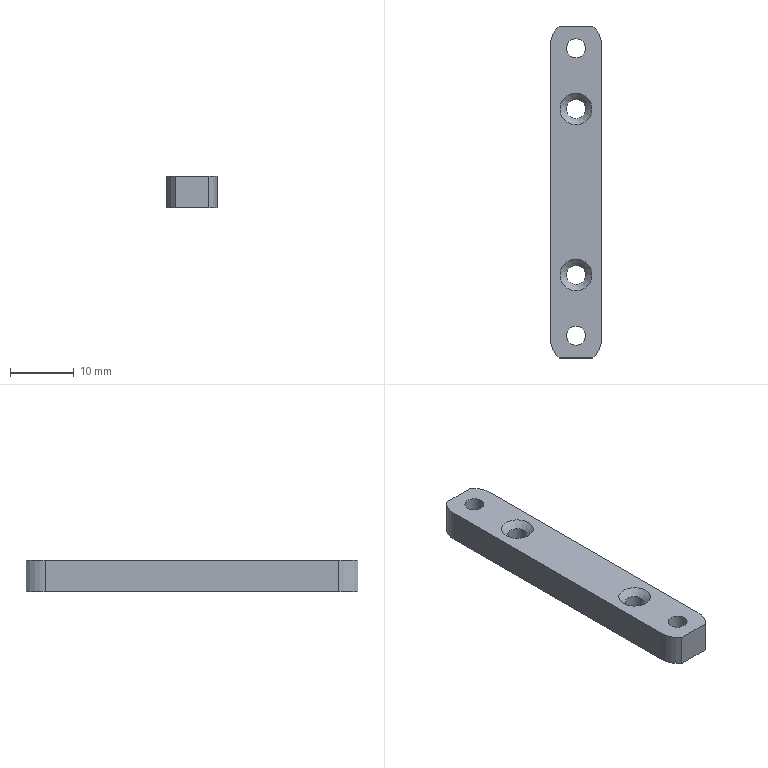Part | STEP file | Wytnij-wyci_gni_cie1_1 | 1 solid | 16 faces | box 8 x 52 x 5 mm | volume 1902 mm3 | cylinder 8 | plane 6 | cone 2 | commonest cylinder face diameters 3 x4 7.98 x4
STEP:
#1=CARTESIAN_POINT('',(0.,0.,0.));
#2=DIRECTION('',(0.,0.,1.));
#3=DIRECTION('',(1.,0.,0.));
#4=AXIS2_PLACEMENT_3D('',#1,#2,#3);
#5=CARTESIAN_POINT('',(-65.244,65.807,-118.498));
#6=VERTEX_POINT('',#5);
#7=CARTESIAN_POINT('',(-63.744,65.807,-118.498));
#8=DIRECTION('',(0.,0.,-1.));
#9=DIRECTION('',(-1.,0.,0.));
#10=AXIS2_PLACEMENT_3D('',#7,#8,#9);
#11=CIRCLE('',#10,1.5);
#12=CARTESIAN_POINT('',(-63.744,65.807,-118.498));
#13=DIRECTION('',(0.,0.,-1.));
#14=DIRECTION('',(-1.,0.,0.));
#15=AXIS2_PLACEMENT_3D('',#12,#13,#14);
#16=CYLINDRICAL_SURFACE('',#15,1.5);
#17=CARTESIAN_POINT('',(0.,0.));
#18=DIRECTION('',(1.,0.));
#19=VECTOR('',#18,1.);
#20=LINE('',#17,#19);
#21=(GEOMETRIC_REPRESENTATION_CONTEXT(2)PARAMETRIC_REPRESENTATION_CONTEXT()REPRESENTATION_CONTEXT('',''));
#22=DEFINITIONAL_REPRESENTATION('',(#20),#21);
#23=PCURVE('',#16,#22);
#24=CARTESIAN_POINT('',(-63.744,88.307,-118.498));
#25=DIRECTION('',(0.,0.,1.));
#26=DIRECTION('',(1.,0.,0.));
#27=AXIS2_PLACEMENT_3D('',#24,#25,#26);
#28=PLANE('',#27);
#29=CARTESIAN_POINT('',(-1.5,-22.5));
#30=CARTESIAN_POINT('',(-1.5,-19.902));
#31=CARTESIAN_POINT('',(0.75,-21.201));
#32=CARTESIAN_POINT('',(3.,-22.5));
#33=CARTESIAN_POINT('',(0.75,-23.799));
#34=CARTESIAN_POINT('',(-1.5,-25.098));
#35=CARTESIAN_POINT('',(-1.5,-22.5));
#36=(BOUNDED_CURVE()B_SPLINE_CURVE(2,(#29,#30,#31,#32,#33,#34,#35),.UNSPECIFIED.,.T.,.F.)B_SPLINE_CURVE_WITH_KNOTS((1,2,2,2,2,1),(-2.094,0.,2.094,4.189,6.283,8.378),.UNSPECIFIED.)CURVE()GEOMETRIC_REPRESENTATION_ITEM()RATIONAL_B_SPLINE_CURVE((1.,0.5,1.,0.5,1.,0.5,1.))REPRESENTATION_ITEM(''));
#37=(GEOMETRIC_REPRESENTATION_CONTEXT(2)PARAMETRIC_REPRESENTATION_CONTEXT()REPRESENTATION_CONTEXT('',''));
#38=DEFINITIONAL_REPRESENTATION('',(#36),#37);
#39=PCURVE('',#28,#38);
#40=SURFACE_CURVE('',#11,(#23,#39),.PCURVE_S1.);
#41=EDGE_CURVE('',#6,#6,#40,.T.);
#42=ORIENTED_EDGE('',*,*,#41,.T.);
#43=CARTESIAN_POINT('',(-65.244,65.807,-123.498));
#44=VERTEX_POINT('',#43);
#45=CARTESIAN_POINT('',(-65.244,65.807,-123.498));
#46=DIRECTION('',(0.,0.,1.));
#47=VECTOR('',#46,1.);
#48=LINE('',#45,#47);
#49=CARTESIAN_POINT('',(6.283,5.));
#50=DIRECTION('',(0.,-1.));
#51=VECTOR('',#50,1.);
#52=LINE('',#49,#51);
#53=(GEOMETRIC_REPRESENTATION_CONTEXT(2)PARAMETRIC_REPRESENTATION_CONTEXT()REPRESENTATION_CONTEXT('',''));
#54=DEFINITIONAL_REPRESENTATION('',(#52),#53);
#55=PCURVE('',#16,#54);
#56=CARTESIAN_POINT('',(0.,5.));
#57=DIRECTION('',(0.,-1.));
#58=VECTOR('',#57,1.);
#59=LINE('',#56,#58);
#60=(GEOMETRIC_REPRESENTATION_CONTEXT(2)PARAMETRIC_REPRESENTATION_CONTEXT()REPRESENTATION_CONTEXT('',''));
#61=DEFINITIONAL_REPRESENTATION('',(#59),#60);
#62=PCURVE('',#16,#61);
#63=SEAM_CURVE('',#48,(#55,#62),.PCURVE_S1.);
#64=EDGE_CURVE('',#44,#6,#63,.T.);
#65=ORIENTED_EDGE('',*,*,#64,.F.);
#66=CARTESIAN_POINT('',(-63.744,65.807,-123.498));
#67=DIRECTION('',(0.,0.,-1.));
#68=DIRECTION('',(-1.,0.,0.));
#69=AXIS2_PLACEMENT_3D('',#66,#67,#68);
#70=CIRCLE('',#69,1.5);
#71=CARTESIAN_POINT('',(0.,5.));
#72=DIRECTION('',(1.,0.));
#73=VECTOR('',#72,1.);
#74=LINE('',#71,#73);
#75=(GEOMETRIC_REPRESENTATION_CONTEXT(2)PARAMETRIC_REPRESENTATION_CONTEXT()REPRESENTATION_CONTEXT('',''));
#76=DEFINITIONAL_REPRESENTATION('',(#74),#75);
#77=PCURVE('',#16,#76);
#78=CARTESIAN_POINT('',(-63.744,88.307,-123.498));
#79=DIRECTION('',(0.,0.,1.));
#80=DIRECTION('',(1.,0.,0.));
#81=AXIS2_PLACEMENT_3D('',#78,#79,#80);
#82=PLANE('',#81);
#83=CARTESIAN_POINT('',(-1.5,-22.5));
#84=CARTESIAN_POINT('',(-1.5,-19.902));
#85=CARTESIAN_POINT('',(0.75,-21.201));
#86=CARTESIAN_POINT('',(3.,-22.5));
#87=CARTESIAN_POINT('',(0.75,-23.799));
#88=CARTESIAN_POINT('',(-1.5,-25.098));
#89=CARTESIAN_POINT('',(-1.5,-22.5));
#90=(BOUNDED_CURVE()B_SPLINE_CURVE(2,(#83,#84,#85,#86,#87,#88,#89),.UNSPECIFIED.,.T.,.F.)B_SPLINE_CURVE_WITH_KNOTS((1,2,2,2,2,1),(-2.094,0.,2.094,4.189,6.283,8.378),.UNSPECIFIED.)CURVE()GEOMETRIC_REPRESENTATION_ITEM()RATIONAL_B_SPLINE_CURVE((1.,0.5,1.,0.5,1.,0.5,1.))REPRESENTATION_ITEM(''));
#91=(GEOMETRIC_REPRESENTATION_CONTEXT(2)PARAMETRIC_REPRESENTATION_CONTEXT()REPRESENTATION_CONTEXT('',''));
#92=DEFINITIONAL_REPRESENTATION('',(#90),#91);
#93=PCURVE('',#82,#92);
#94=SURFACE_CURVE('',#70,(#77,#93),.PCURVE_S1.);
#95=EDGE_CURVE('',#44,#44,#94,.T.);
#96=ORIENTED_EDGE('',*,*,#95,.F.);
#97=ORIENTED_EDGE('',*,*,#64,.T.);
#98=EDGE_LOOP('',(#42,#65,#96,#97));
#99=FACE_BOUND('',#98,.F.);
#100=ADVANCED_FACE('',(#99),#16,.F.);
#101=CARTESIAN_POINT('',(-65.244,110.807,-118.498));
#102=VERTEX_POINT('',#101);
#103=CARTESIAN_POINT('',(-63.744,110.807,-118.498));
#104=DIRECTION('',(0.,0.,-1.));
#105=DIRECTION('',(-1.,0.,0.));
#106=AXIS2_PLACEMENT_3D('',#103,#104,#105);
#107=CIRCLE('',#106,1.5);
#108=CARTESIAN_POINT('',(-63.744,110.807,-118.498));
#109=DIRECTION('',(0.,0.,-1.));
#110=DIRECTION('',(-1.,0.,0.));
#111=AXIS2_PLACEMENT_3D('',#108,#109,#110);
#112=CYLINDRICAL_SURFACE('',#111,1.5);
#113=CARTESIAN_POINT('',(0.,0.));
#114=DIRECTION('',(1.,0.));
#115=VECTOR('',#114,1.);
#116=LINE('',#113,#115);
#117=(GEOMETRIC_REPRESENTATION_CONTEXT(2)PARAMETRIC_REPRESENTATION_CONTEXT()REPRESENTATION_CONTEXT('',''));
#118=DEFINITIONAL_REPRESENTATION('',(#116),#117);
#119=PCURVE('',#112,#118);
#120=CARTESIAN_POINT('',(-1.5,22.5));
#121=CARTESIAN_POINT('',(-1.5,25.098));
#122=CARTESIAN_POINT('',(0.75,23.799));
#123=CARTESIAN_POINT('',(3.,22.5));
#124=CARTESIAN_POINT('',(0.75,21.201));
#125=CARTESIAN_POINT('',(-1.5,19.902));
#126=CARTESIAN_POINT('',(-1.5,22.5));
#127=(BOUNDED_CURVE()B_SPLINE_CURVE(2,(#120,#121,#122,#123,#124,#125,#126),.UNSPECIFIED.,.T.,.F.)B_SPLINE_CURVE_WITH_KNOTS((1,2,2,2,2,1),(-2.094,0.,2.094,4.189,6.283,8.378),.UNSPECIFIED.)CURVE()GEOMETRIC_REPRESENTATION_ITEM()RATIONAL_B_SPLINE_CURVE((1.,0.5,1.,0.5,1.,0.5,1.))REPRESENTATION_ITEM(''));
#128=(GEOMETRIC_REPRESENTATION_CONTEXT(2)PARAMETRIC_REPRESENTATION_CONTEXT()REPRESENTATION_CONTEXT('',''));
#129=DEFINITIONAL_REPRESENTATION('',(#127),#128);
#130=PCURVE('',#28,#129);
#131=SURFACE_CURVE('',#107,(#119,#130),.PCURVE_S1.);
#132=EDGE_CURVE('',#102,#102,#131,.T.);
#133=ORIENTED_EDGE('',*,*,#132,.T.);
#134=CARTESIAN_POINT('',(-65.244,110.807,-123.498));
#135=VERTEX_POINT('',#134);
#136=CARTESIAN_POINT('',(-65.244,110.807,-123.498));
#137=DIRECTION('',(0.,0.,1.));
#138=VECTOR('',#137,1.);
#139=LINE('',#136,#138);
#140=CARTESIAN_POINT('',(6.283,5.));
#141=DIRECTION('',(0.,-1.));
#142=VECTOR('',#141,1.);
#143=LINE('',#140,#142);
#144=(GEOMETRIC_REPRESENTATION_CONTEXT(2)PARAMETRIC_REPRESENTATION_CONTEXT()REPRESENTATION_CONTEXT('',''));
#145=DEFINITIONAL_REPRESENTATION('',(#143),#144);
#146=PCURVE('',#112,#145);
#147=CARTESIAN_POINT('',(0.,5.));
#148=DIRECTION('',(0.,-1.));
#149=VECTOR('',#148,1.);
#150=LINE('',#147,#149);
#151=(GEOMETRIC_REPRESENTATION_CONTEXT(2)PARAMETRIC_REPRESENTATION_CONTEXT()REPRESENTATION_CONTEXT('',''));
#152=DEFINITIONAL_REPRESENTATION('',(#150),#151);
#153=PCURVE('',#112,#152);
#154=SEAM_CURVE('',#139,(#146,#153),.PCURVE_S1.);
#155=EDGE_CURVE('',#135,#102,#154,.T.);
#156=ORIENTED_EDGE('',*,*,#155,.F.);
#157=CARTESIAN_POINT('',(-63.744,110.807,-123.498));
#158=DIRECTION('',(0.,0.,-1.));
#159=DIRECTION('',(-1.,0.,0.));
#160=AXIS2_PLACEMENT_3D('',#157,#158,#159);
#161=CIRCLE('',#160,1.5);
#162=CARTESIAN_POINT('',(0.,5.));
#163=DIRECTION('',(1.,0.));
#164=VECTOR('',#163,1.);
#165=LINE('',#162,#164);
#166=(GEOMETRIC_REPRESENTATION_CONTEXT(2)PARAMETRIC_REPRESENTATION_CONTEXT()REPRESENTATION_CONTEXT('',''));
#167=DEFINITIONAL_REPRESENTATION('',(#165),#166);
#168=PCURVE('',#112,#167);
#169=CARTESIAN_POINT('',(-1.5,22.5));
#170=CARTESIAN_POINT('',(-1.5,25.098));
#171=CARTESIAN_POINT('',(0.75,23.799));
#172=CARTESIAN_POINT('',(3.,22.5));
#173=CARTESIAN_POINT('',(0.75,21.201));
#174=CARTESIAN_POINT('',(-1.5,19.902));
#175=CARTESIAN_POINT('',(-1.5,22.5));
#176=(BOUNDED_CURVE()B_SPLINE_CURVE(2,(#169,#170,#171,#172,#173,#174,#175),.UNSPECIFIED.,.T.,.F.)B_SPLINE_CURVE_WITH_KNOTS((1,2,2,2,2,1),(-2.094,0.,2.094,4.189,6.283,8.378),.UNSPECIFIED.)CURVE()GEOMETRIC_REPRESENTATION_ITEM()RATIONAL_B_SPLINE_CURVE((1.,0.5,1.,0.5,1.,0.5,1.))REPRESENTATION_ITEM(''));
#177=(GEOMETRIC_REPRESENTATION_CONTEXT(2)PARAMETRIC_REPRESENTATION_CONTEXT()REPRESENTATION_CONTEXT('',''));
#178=DEFINITIONAL_REPRESENTATION('',(#176),#177);
#179=PCURVE('',#82,#178);
#180=SURFACE_CURVE('',#161,(#168,#179),.PCURVE_S1.);
#181=EDGE_CURVE('',#135,#135,#180,.T.);
#182=ORIENTED_EDGE('',*,*,#181,.F.);
#183=ORIENTED_EDGE('',*,*,#155,.T.);
#184=EDGE_LOOP('',(#133,#156,#182,#183));
#185=FACE_BOUND('',#184,.F.);
#186=ADVANCED_FACE('',(#185),#112,.F.);
#187=CARTESIAN_POINT('',(-65.244,75.307,-119.498));
#188=VERTEX_POINT('',#187);
#189=CARTESIAN_POINT('',(-62.244,75.307,-119.498));
#190=VERTEX_POINT('',#189);
#191=CARTESIAN_POINT('',(-63.744,75.307,-119.498));
#192=DIRECTION('',(0.,0.,-1.));
#193=DIRECTION('',(1.,0.,0.));
#194=AXIS2_PLACEMENT_3D('',#191,#192,#193);
#195=CIRCLE('',#194,1.5);
#196=CARTESIAN_POINT('',(-63.744,75.307,-119.498));
#197=DIRECTION('',(0.,0.,-1.));
#198=DIRECTION('',(-1.,0.,0.));
#199=AXIS2_PLACEMENT_3D('',#196,#197,#198);
#200=CYLINDRICAL_SURFACE('',#199,1.5);
#201=CARTESIAN_POINT('',(-3.142,0.));
#202=DIRECTION('',(1.,0.));
#203=VECTOR('',#202,1.);
#204=LINE('',#201,#203);
#205=(GEOMETRIC_REPRESENTATION_CONTEXT(2)PARAMETRIC_REPRESENTATION_CONTEXT()REPRESENTATION_CONTEXT('',''));
#206=DEFINITIONAL_REPRESENTATION('',(#204),#205);
#207=PCURVE('',#200,#206);
#208=CARTESIAN_POINT('',(-63.744,75.307,-118.498));
#209=DIRECTION('',(0.,0.,1.));
#210=DIRECTION('',(1.,0.,0.));
#211=AXIS2_PLACEMENT_3D('',#208,#209,#210);
#212=CONICAL_SURFACE('',#211,2.5,0.7854);
#213=CARTESIAN_POINT('',(6.283,-1.));
#214=DIRECTION('',(-1.,0.));
#215=VECTOR('',#214,1.);
#216=LINE('',#213,#215);
#217=(GEOMETRIC_REPRESENTATION_CONTEXT(2)PARAMETRIC_REPRESENTATION_CONTEXT()REPRESENTATION_CONTEXT('',''));
#218=DEFINITIONAL_REPRESENTATION('',(#216),#217);
#219=PCURVE('',#212,#218);
#220=SURFACE_CURVE('',#195,(#207,#219),.PCURVE_S1.);
#221=EDGE_CURVE('',#188,#190,#220,.T.);
#222=ORIENTED_EDGE('',*,*,#221,.T.);
#223=CARTESIAN_POINT('',(-63.744,75.307,-119.498));
#224=DIRECTION('',(0.,0.,-1.));
#225=DIRECTION('',(1.,0.,0.));
#226=AXIS2_PLACEMENT_3D('',#223,#224,#225);
#227=CIRCLE('',#226,1.5);
#228=CARTESIAN_POINT('',(3.142,0.));
#229=DIRECTION('',(1.,0.));
#230=VECTOR('',#229,1.);
#231=LINE('',#228,#230);
#232=(GEOMETRIC_REPRESENTATION_CONTEXT(2)PARAMETRIC_REPRESENTATION_CONTEXT()REPRESENTATION_CONTEXT('',''));
#233=DEFINITIONAL_REPRESENTATION('',(#231),#232);
#234=PCURVE('',#200,#233);
#235=CARTESIAN_POINT('',(6.283,-1.));
#236=DIRECTION('',(-1.,0.));
#237=VECTOR('',#236,1.);
#238=LINE('',#235,#237);
#239=(GEOMETRIC_REPRESENTATION_CONTEXT(2)PARAMETRIC_REPRESENTATION_CONTEXT()REPRESENTATION_CONTEXT('',''));
#240=DEFINITIONAL_REPRESENTATION('',(#238),#239);
#241=PCURVE('',#212,#240);
#242=SURFACE_CURVE('',#227,(#234,#241),.PCURVE_S1.);
#243=EDGE_CURVE('',#190,#188,#242,.T.);
#244=ORIENTED_EDGE('',*,*,#243,.T.);
#245=CARTESIAN_POINT('',(-65.244,75.307,-123.498));
#246=VERTEX_POINT('',#245);
#247=CARTESIAN_POINT('',(-65.244,75.307,-123.498));
#248=DIRECTION('',(0.,0.,1.));
#249=VECTOR('',#248,1.);
#250=LINE('',#247,#249);
#251=CARTESIAN_POINT('',(6.283,4.));
#252=DIRECTION('',(0.,-1.));
#253=VECTOR('',#252,1.);
#254=LINE('',#251,#253);
#255=(GEOMETRIC_REPRESENTATION_CONTEXT(2)PARAMETRIC_REPRESENTATION_CONTEXT()REPRESENTATION_CONTEXT('',''));
#256=DEFINITIONAL_REPRESENTATION('',(#254),#255);
#257=PCURVE('',#200,#256);
#258=CARTESIAN_POINT('',(0.,4.));
#259=DIRECTION('',(0.,-1.));
#260=VECTOR('',#259,1.);
#261=LINE('',#258,#260);
#262=(GEOMETRIC_REPRESENTATION_CONTEXT(2)PARAMETRIC_REPRESENTATION_CONTEXT()REPRESENTATION_CONTEXT('',''));
#263=DEFINITIONAL_REPRESENTATION('',(#261),#262);
#264=PCURVE('',#200,#263);
#265=SEAM_CURVE('',#250,(#257,#264),.PCURVE_S1.);
#266=EDGE_CURVE('',#246,#188,#265,.T.);
#267=ORIENTED_EDGE('',*,*,#266,.F.);
#268=CARTESIAN_POINT('',(-63.744,75.307,-123.498));
#269=DIRECTION('',(0.,0.,-1.));
#270=DIRECTION('',(-1.,0.,0.));
#271=AXIS2_PLACEMENT_3D('',#268,#269,#270);
#272=CIRCLE('',#271,1.5);
#273=CARTESIAN_POINT('',(0.,4.));
#274=DIRECTION('',(1.,0.));
#275=VECTOR('',#274,1.);
#276=LINE('',#273,#275);
#277=(GEOMETRIC_REPRESENTATION_CONTEXT(2)PARAMETRIC_REPRESENTATION_CONTEXT()REPRESENTATION_CONTEXT('',''));
#278=DEFINITIONAL_REPRESENTATION('',(#276),#277);
#279=PCURVE('',#200,#278);
#280=CARTESIAN_POINT('',(-1.5,-13.));
#281=CARTESIAN_POINT('',(-1.5,-10.402));
#282=CARTESIAN_POINT('',(0.75,-11.701));
#283=CARTESIAN_POINT('',(3.,-13.));
#284=CARTESIAN_POINT('',(0.75,-14.299));
#285=CARTESIAN_POINT('',(-1.5,-15.598));
#286=CARTESIAN_POINT('',(-1.5,-13.));
#287=(BOUNDED_CURVE()B_SPLINE_CURVE(2,(#280,#281,#282,#283,#284,#285,#286),.UNSPECIFIED.,.T.,.F.)B_SPLINE_CURVE_WITH_KNOTS((1,2,2,2,2,1),(-2.094,0.,2.094,4.189,6.283,8.378),.UNSPECIFIED.)CURVE()GEOMETRIC_REPRESENTATION_ITEM()RATIONAL_B_SPLINE_CURVE((1.,0.5,1.,0.5,1.,0.5,1.))REPRESENTATION_ITEM(''));
#288=(GEOMETRIC_REPRESENTATION_CONTEXT(2)PARAMETRIC_REPRESENTATION_CONTEXT()REPRESENTATION_CONTEXT('',''));
#289=DEFINITIONAL_REPRESENTATION('',(#287),#288);
#290=PCURVE('',#82,#289);
#291=SURFACE_CURVE('',#272,(#279,#290),.PCURVE_S1.);
#292=EDGE_CURVE('',#246,#246,#291,.T.);
#293=ORIENTED_EDGE('',*,*,#292,.F.);
#294=ORIENTED_EDGE('',*,*,#266,.T.);
#295=EDGE_LOOP('',(#222,#244,#267,#293,#294));
#296=FACE_BOUND('',#295,.F.);
#297=ADVANCED_FACE('',(#296),#200,.F.);
#298=CARTESIAN_POINT('',(-65.244,101.307,-119.498));
#299=VERTEX_POINT('',#298);
#300=CARTESIAN_POINT('',(-62.244,101.307,-119.498));
#301=VERTEX_POINT('',#300);
#302=CARTESIAN_POINT('',(-63.744,101.307,-119.498));
#303=DIRECTION('',(0.,0.,-1.));
#304=DIRECTION('',(1.,0.,0.));
#305=AXIS2_PLACEMENT_3D('',#302,#303,#304);
#306=CIRCLE('',#305,1.5);
#307=CARTESIAN_POINT('',(-63.744,101.307,-119.498));
#308=DIRECTION('',(0.,0.,-1.));
#309=DIRECTION('',(-1.,0.,0.));
#310=AXIS2_PLACEMENT_3D('',#307,#308,#309);
#311=CYLINDRICAL_SURFACE('',#310,1.5);
#312=CARTESIAN_POINT('',(-3.142,0.));
#313=DIRECTION('',(1.,0.));
#314=VECTOR('',#313,1.);
#315=LINE('',#312,#314);
#316=(GEOMETRIC_REPRESENTATION_CONTEXT(2)PARAMETRIC_REPRESENTATION_CONTEXT()REPRESENTATION_CONTEXT('',''));
#317=DEFINITIONAL_REPRESENTATION('',(#315),#316);
#318=PCURVE('',#311,#317);
#319=CARTESIAN_POINT('',(-63.744,101.307,-118.498));
#320=DIRECTION('',(0.,0.,1.));
#321=DIRECTION('',(1.,0.,0.));
#322=AXIS2_PLACEMENT_3D('',#319,#320,#321);
#323=CONICAL_SURFACE('',#322,2.5,0.7854);
#324=CARTESIAN_POINT('',(6.283,-1.));
#325=DIRECTION('',(-1.,0.));
#326=VECTOR('',#325,1.);
#327=LINE('',#324,#326);
#328=(GEOMETRIC_REPRESENTATION_CONTEXT(2)PARAMETRIC_REPRESENTATION_CONTEXT()REPRESENTATION_CONTEXT('',''));
#329=DEFINITIONAL_REPRESENTATION('',(#327),#328);
#330=PCURVE('',#323,#329);
#331=SURFACE_CURVE('',#306,(#318,#330),.PCURVE_S1.);
#332=EDGE_CURVE('',#299,#301,#331,.T.);
#333=ORIENTED_EDGE('',*,*,#332,.T.);
#334=CARTESIAN_POINT('',(-63.744,101.307,-119.498));
#335=DIRECTION('',(0.,0.,-1.));
#336=DIRECTION('',(1.,0.,0.));
#337=AXIS2_PLACEMENT_3D('',#334,#335,#336);
#338=CIRCLE('',#337,1.5);
#339=CARTESIAN_POINT('',(3.142,0.));
#340=DIRECTION('',(1.,0.));
#341=VECTOR('',#340,1.);
#342=LINE('',#339,#341);
#343=(GEOMETRIC_REPRESENTATION_CONTEXT(2)PARAMETRIC_REPRESENTATION_CONTEXT()REPRESENTATION_CONTEXT('',''));
#344=DEFINITIONAL_REPRESENTATION('',(#342),#343);
#345=PCURVE('',#311,#344);
#346=CARTESIAN_POINT('',(6.283,-1.));
#347=DIRECTION('',(-1.,0.));
#348=VECTOR('',#347,1.);
#349=LINE('',#346,#348);
#350=(GEOMETRIC_REPRESENTATION_CONTEXT(2)PARAMETRIC_REPRESENTATION_CONTEXT()REPRESENTATION_CONTEXT('',''));
#351=DEFINITIONAL_REPRESENTATION('',(#349),#350);
#352=PCURVE('',#323,#351);
#353=SURFACE_CURVE('',#338,(#345,#352),.PCURVE_S1.);
#354=EDGE_CURVE('',#301,#299,#353,.T.);
#355=ORIENTED_EDGE('',*,*,#354,.T.);
#356=CARTESIAN_POINT('',(-65.244,101.307,-123.498));
#357=VERTEX_POINT('',#356);
#358=CARTESIAN_POINT('',(-65.244,101.307,-123.498));
#359=DIRECTION('',(0.,0.,1.));
#360=VECTOR('',#359,1.);
#361=LINE('',#358,#360);
#362=CARTESIAN_POINT('',(6.283,4.));
#363=DIRECTION('',(0.,-1.));
#364=VECTOR('',#363,1.);
#365=LINE('',#362,#364);
#366=(GEOMETRIC_REPRESENTATION_CONTEXT(2)PARAMETRIC_REPRESENTATION_CONTEXT()REPRESENTATION_CONTEXT('',''));
#367=DEFINITIONAL_REPRESENTATION('',(#365),#366);
#368=PCURVE('',#311,#367);
#369=CARTESIAN_POINT('',(0.,4.));
#370=DIRECTION('',(0.,-1.));
#371=VECTOR('',#370,1.);
#372=LINE('',#369,#371);
#373=(GEOMETRIC_REPRESENTATION_CONTEXT(2)PARAMETRIC_REPRESENTATION_CONTEXT()REPRESENTATION_CONTEXT('',''));
#374=DEFINITIONAL_REPRESENTATION('',(#372),#373);
#375=PCURVE('',#311,#374);
#376=SEAM_CURVE('',#361,(#368,#375),.PCURVE_S1.);
#377=EDGE_CURVE('',#357,#299,#376,.T.);
#378=ORIENTED_EDGE('',*,*,#377,.F.);
#379=CARTESIAN_POINT('',(-63.744,101.307,-123.498));
#380=DIRECTION('',(0.,0.,-1.));
#381=DIRECTION('',(-1.,0.,0.));
#382=AXIS2_PLACEMENT_3D('',#379,#380,#381);
#383=CIRCLE('',#382,1.5);
#384=CARTESIAN_POINT('',(0.,4.));
#385=DIRECTION('',(1.,0.));
#386=VECTOR('',#385,1.);
#387=LINE('',#384,#386);
#388=(GEOMETRIC_REPRESENTATION_CONTEXT(2)PARAMETRIC_REPRESENTATION_CONTEXT()REPRESENTATION_CONTEXT('',''));
#389=DEFINITIONAL_REPRESENTATION('',(#387),#388);
#390=PCURVE('',#311,#389);
#391=CARTESIAN_POINT('',(-1.5,13.));
#392=CARTESIAN_POINT('',(-1.5,15.598));
#393=CARTESIAN_POINT('',(0.75,14.299));
#394=CARTESIAN_POINT('',(3.,13.));
#395=CARTESIAN_POINT('',(0.75,11.701));
#396=CARTESIAN_POINT('',(-1.5,10.402));
#397=CARTESIAN_POINT('',(-1.5,13.));
#398=(BOUNDED_CURVE()B_SPLINE_CURVE(2,(#391,#392,#393,#394,#395,#396,#397),.UNSPECIFIED.,.T.,.F.)B_SPLINE_CURVE_WITH_KNOTS((1,2,2,2,2,1),(-2.094,0.,2.094,4.189,6.283,8.378),.UNSPECIFIED.)CURVE()GEOMETRIC_REPRESENTATION_ITEM()RATIONAL_B_SPLINE_CURVE((1.,0.5,1.,0.5,1.,0.5,1.))REPRESENTATION_ITEM(''));
#399=(GEOMETRIC_REPRESENTATION_CONTEXT(2)PARAMETRIC_REPRESENTATION_CONTEXT()REPRESENTATION_CONTEXT('',''));
#400=DEFINITIONAL_REPRESENTATION('',(#398),#399);
#401=PCURVE('',#82,#400);
#402=SURFACE_CURVE('',#383,(#390,#401),.PCURVE_S1.);
#403=EDGE_CURVE('',#357,#357,#402,.T.);
#404=ORIENTED_EDGE('',*,*,#403,.F.);
#405=ORIENTED_EDGE('',*,*,#377,.T.);
#406=EDGE_LOOP('',(#333,#355,#378,#404,#405));
#407=FACE_BOUND('',#406,.F.);
#408=ADVANCED_FACE('',(#407),#311,.F.);
#409=ORIENTED_EDGE('',*,*,#221,.F.);
#410=ORIENTED_EDGE('',*,*,#243,.F.);
#411=CARTESIAN_POINT('',(-61.244,75.307,-118.498));
#412=VERTEX_POINT('',#411);
#413=CARTESIAN_POINT('',(-61.244,75.307,-118.498));
#414=DIRECTION('',(-0.7071,0.,-0.7071));
#415=VECTOR('',#414,1.);
#416=LINE('',#413,#415);
#417=CARTESIAN_POINT('',(6.283,0.));
#418=DIRECTION('',(0.,-1.));
#419=VECTOR('',#418,1.);
#420=LINE('',#417,#419);
#421=(GEOMETRIC_REPRESENTATION_CONTEXT(2)PARAMETRIC_REPRESENTATION_CONTEXT()REPRESENTATION_CONTEXT('',''));
#422=DEFINITIONAL_REPRESENTATION('',(#420),#421);
#423=PCURVE('',#212,#422);
#424=CARTESIAN_POINT('',(0.,0.));
#425=DIRECTION('',(0.,-1.));
#426=VECTOR('',#425,1.);
#427=LINE('',#424,#426);
#428=(GEOMETRIC_REPRESENTATION_CONTEXT(2)PARAMETRIC_REPRESENTATION_CONTEXT()REPRESENTATION_CONTEXT('',''));
#429=DEFINITIONAL_REPRESENTATION('',(#427),#428);
#430=PCURVE('',#212,#429);
#431=SEAM_CURVE('',#416,(#423,#430),.PCURVE_S1.);
#432=EDGE_CURVE('',#412,#190,#431,.T.);
#433=ORIENTED_EDGE('',*,*,#432,.F.);
#434=CARTESIAN_POINT('',(-63.744,75.307,-118.498));
#435=DIRECTION('',(0.,0.,-1.));
#436=DIRECTION('',(1.,0.,0.));
#437=AXIS2_PLACEMENT_3D('',#434,#435,#436);
#438=CIRCLE('',#437,2.5);
#439=CARTESIAN_POINT('',(6.283,0.));
#440=DIRECTION('',(-1.,0.));
#441=VECTOR('',#440,1.);
#442=LINE('',#439,#441);
#443=(GEOMETRIC_REPRESENTATION_CONTEXT(2)PARAMETRIC_REPRESENTATION_CONTEXT()REPRESENTATION_CONTEXT('',''));
#444=DEFINITIONAL_REPRESENTATION('',(#442),#443);
#445=PCURVE('',#212,#444);
#446=CARTESIAN_POINT('',(2.5,-13.));
#447=CARTESIAN_POINT('',(2.5,-17.33));
#448=CARTESIAN_POINT('',(-1.25,-15.165));
#449=CARTESIAN_POINT('',(-5.,-13.));
#450=CARTESIAN_POINT('',(-1.25,-10.835));
#451=CARTESIAN_POINT('',(2.5,-8.67));
#452=CARTESIAN_POINT('',(2.5,-13.));
#453=(BOUNDED_CURVE()B_SPLINE_CURVE(2,(#446,#447,#448,#449,#450,#451,#452),.UNSPECIFIED.,.T.,.F.)B_SPLINE_CURVE_WITH_KNOTS((1,2,2,2,2,1),(-2.094,0.,2.094,4.189,6.283,8.378),.UNSPECIFIED.)CURVE()GEOMETRIC_REPRESENTATION_ITEM()RATIONAL_B_SPLINE_CURVE((1.,0.5,1.,0.5,1.,0.5,1.))REPRESENTATION_ITEM(''));
#454=(GEOMETRIC_REPRESENTATION_CONTEXT(2)PARAMETRIC_REPRESENTATION_CONTEXT()REPRESENTATION_CONTEXT('',''));
#455=DEFINITIONAL_REPRESENTATION('',(#453),#454);
#456=PCURVE('',#28,#455);
#457=SURFACE_CURVE('',#438,(#445,#456),.PCURVE_S1.);
#458=EDGE_CURVE('',#412,#412,#457,.T.);
#459=ORIENTED_EDGE('',*,*,#458,.T.);
#460=ORIENTED_EDGE('',*,*,#432,.T.);
#461=EDGE_LOOP('',(#409,#410,#433,#459,#460));
#462=FACE_BOUND('',#461,.F.);
#463=ADVANCED_FACE('',(#462),#212,.F.);
#464=ORIENTED_EDGE('',*,*,#332,.F.);
#465=ORIENTED_EDGE('',*,*,#354,.F.);
#466=CARTESIAN_POINT('',(-61.244,101.307,-118.498));
#467=VERTEX_POINT('',#466);
#468=CARTESIAN_POINT('',(-61.244,101.307,-118.498));
#469=DIRECTION('',(-0.7071,0.,-0.7071));
#470=VECTOR('',#469,1.);
#471=LINE('',#468,#470);
#472=CARTESIAN_POINT('',(6.283,0.));
#473=DIRECTION('',(0.,-1.));
#474=VECTOR('',#473,1.);
#475=LINE('',#472,#474);
#476=(GEOMETRIC_REPRESENTATION_CONTEXT(2)PARAMETRIC_REPRESENTATION_CONTEXT()REPRESENTATION_CONTEXT('',''));
#477=DEFINITIONAL_REPRESENTATION('',(#475),#476);
#478=PCURVE('',#323,#477);
#479=CARTESIAN_POINT('',(0.,0.));
#480=DIRECTION('',(0.,-1.));
#481=VECTOR('',#480,1.);
#482=LINE('',#479,#481);
#483=(GEOMETRIC_REPRESENTATION_CONTEXT(2)PARAMETRIC_REPRESENTATION_CONTEXT()REPRESENTATION_CONTEXT('',''));
#484=DEFINITIONAL_REPRESENTATION('',(#482),#483);
#485=PCURVE('',#323,#484);
#486=SEAM_CURVE('',#471,(#478,#485),.PCURVE_S1.);
#487=EDGE_CURVE('',#467,#301,#486,.T.);
#488=ORIENTED_EDGE('',*,*,#487,.F.);
#489=CARTESIAN_POINT('',(-63.744,101.307,-118.498));
#490=DIRECTION('',(0.,0.,-1.));
#491=DIRECTION('',(1.,0.,0.));
#492=AXIS2_PLACEMENT_3D('',#489,#490,#491);
#493=CIRCLE('',#492,2.5);
#494=CARTESIAN_POINT('',(6.283,0.));
#495=DIRECTION('',(-1.,0.));
#496=VECTOR('',#495,1.);
#497=LINE('',#494,#496);
#498=(GEOMETRIC_REPRESENTATION_CONTEXT(2)PARAMETRIC_REPRESENTATION_CONTEXT()REPRESENTATION_CONTEXT('',''));
#499=DEFINITIONAL_REPRESENTATION('',(#497),#498);
#500=PCURVE('',#323,#499);
#501=CARTESIAN_POINT('',(2.5,13.));
#502=CARTESIAN_POINT('',(2.5,8.67));
#503=CARTESIAN_POINT('',(-1.25,10.835));
#504=CARTESIAN_POINT('',(-5.,13.));
#505=CARTESIAN_POINT('',(-1.25,15.165));
#506=CARTESIAN_POINT('',(2.5,17.33));
#507=CARTESIAN_POINT('',(2.5,13.));
#508=(BOUNDED_CURVE()B_SPLINE_CURVE(2,(#501,#502,#503,#504,#505,#506,#507),.UNSPECIFIED.,.T.,.F.)B_SPLINE_CURVE_WITH_KNOTS((1,2,2,2,2,1),(-2.094,0.,2.094,4.189,6.283,8.378),.UNSPECIFIED.)CURVE()GEOMETRIC_REPRESENTATION_ITEM()RATIONAL_B_SPLINE_CURVE((1.,0.5,1.,0.5,1.,0.5,1.))REPRESENTATION_ITEM(''));
#509=(GEOMETRIC_REPRESENTATION_CONTEXT(2)PARAMETRIC_REPRESENTATION_CONTEXT()REPRESENTATION_CONTEXT('',''));
#510=DEFINITIONAL_REPRESENTATION('',(#508),#509);
#511=PCURVE('',#28,#510);
#512=SURFACE_CURVE('',#493,(#500,#511),.PCURVE_S1.);
#513=EDGE_CURVE('',#467,#467,#512,.T.);
#514=ORIENTED_EDGE('',*,*,#513,.T.);
#515=ORIENTED_EDGE('',*,*,#487,.T.);
#516=EDGE_LOOP('',(#464,#465,#488,#514,#515));
#517=FACE_BOUND('',#516,.F.);
#518=ADVANCED_FACE('',(#517),#323,.F.);
#519=ORIENTED_EDGE('',*,*,#95,.F.);
#520=EDGE_LOOP('',(#519));
#521=FACE_BOUND('',#520,.T.);
#522=ORIENTED_EDGE('',*,*,#181,.F.);
#523=EDGE_LOOP('',(#522));
#524=FACE_BOUND('',#523,.T.);
#525=ORIENTED_EDGE('',*,*,#292,.F.);
#526=EDGE_LOOP('',(#525));
#527=FACE_BOUND('',#526,.T.);
#528=ORIENTED_EDGE('',*,*,#403,.F.);
#529=EDGE_LOOP('',(#528));
#530=FACE_BOUND('',#529,.T.);
#531=CARTESIAN_POINT('',(-67.744,65.297,-123.498));
#532=VERTEX_POINT('',#531);
#533=CARTESIAN_POINT('',(-66.396,62.307,-123.498));
#534=VERTEX_POINT('',#533);
#535=CARTESIAN_POINT('',(-63.754,65.297,-123.498));
#536=DIRECTION('',(0.,0.,1.));
#537=DIRECTION('',(-1.,0.,0.));
#538=AXIS2_PLACEMENT_3D('',#535,#536,#537);
#539=CIRCLE('',#538,3.99);
#540=CARTESIAN_POINT('',(-0.01,-23.01));
#541=DIRECTION('',(-1.,0.));
#542=AXIS2_PLACEMENT_2D('',#540,#541);
#543=CIRCLE('',#542,3.99);
#544=(GEOMETRIC_REPRESENTATION_CONTEXT(2)PARAMETRIC_REPRESENTATION_CONTEXT()REPRESENTATION_CONTEXT('',''));
#545=DEFINITIONAL_REPRESENTATION('',(#543),#544);
#546=PCURVE('',#82,#545);
#547=CARTESIAN_POINT('',(-63.754,65.297,-118.498));
#548=DIRECTION('',(0.,0.,-1.));
#549=DIRECTION('',(-1.,0.,0.));
#550=AXIS2_PLACEMENT_3D('',#547,#548,#549);
#551=CYLINDRICAL_SURFACE('',#550,3.99);
#552=CARTESIAN_POINT('',(6.283,5.));
#553=DIRECTION('',(-1.,0.));
#554=VECTOR('',#553,1.);
#555=LINE('',#552,#554);
#556=(GEOMETRIC_REPRESENTATION_CONTEXT(2)PARAMETRIC_REPRESENTATION_CONTEXT()REPRESENTATION_CONTEXT('',''));
#557=DEFINITIONAL_REPRESENTATION('',(#555),#556);
#558=PCURVE('',#551,#557);
#559=SURFACE_CURVE('',#539,(#546,#558),.PCURVE_S1.);
#560=EDGE_CURVE('',#532,#534,#559,.T.);
#561=ORIENTED_EDGE('',*,*,#560,.F.);
#562=CARTESIAN_POINT('',(-67.744,111.317,-123.498));
#563=VERTEX_POINT('',#562);
#564=CARTESIAN_POINT('',(-67.744,111.317,-123.498));
#565=DIRECTION('',(0.,-1.,0.));
#566=VECTOR('',#565,1.);
#567=LINE('',#564,#566);
#568=CARTESIAN_POINT('',(-4.,23.01));
#569=DIRECTION('',(0.,-1.));
#570=VECTOR('',#569,1.);
#571=LINE('',#568,#570);
#572=(GEOMETRIC_REPRESENTATION_CONTEXT(2)PARAMETRIC_REPRESENTATION_CONTEXT()REPRESENTATION_CONTEXT('',''));
#573=DEFINITIONAL_REPRESENTATION('',(#571),#572);
#574=PCURVE('',#82,#573);
#575=CARTESIAN_POINT('',(-67.744,88.307,-120.998));
#576=DIRECTION('',(1.,0.,0.));
#577=DIRECTION('',(0.,1.,0.));
#578=AXIS2_PLACEMENT_3D('',#575,#576,#577);
#579=PLANE('',#578);
#580=CARTESIAN_POINT('',(23.01,-2.5));
#581=DIRECTION('',(-1.,0.));
#582=VECTOR('',#581,1.);
#583=LINE('',#580,#582);
#584=(GEOMETRIC_REPRESENTATION_CONTEXT(2)PARAMETRIC_REPRESENTATION_CONTEXT()REPRESENTATION_CONTEXT('',''));
#585=DEFINITIONAL_REPRESENTATION('',(#583),#584);
#586=PCURVE('',#579,#585);
#587=SURFACE_CURVE('',#567,(#574,#586),.PCURVE_S1.);
#588=EDGE_CURVE('',#563,#532,#587,.T.);
#589=ORIENTED_EDGE('',*,*,#588,.F.);
#590=CARTESIAN_POINT('',(-66.396,114.307,-123.498));
#591=VERTEX_POINT('',#590);
#592=CARTESIAN_POINT('',(-63.754,111.317,-123.498));
#593=DIRECTION('',(0.,0.,1.));
#594=DIRECTION('',(-1.,0.,0.));
#595=AXIS2_PLACEMENT_3D('',#592,#593,#594);
#596=CIRCLE('',#595,3.99);
#597=CARTESIAN_POINT('',(-0.01,23.01));
#598=DIRECTION('',(-1.,0.));
#599=AXIS2_PLACEMENT_2D('',#597,#598);
#600=CIRCLE('',#599,3.99);
#601=(GEOMETRIC_REPRESENTATION_CONTEXT(2)PARAMETRIC_REPRESENTATION_CONTEXT()REPRESENTATION_CONTEXT('',''));
#602=DEFINITIONAL_REPRESENTATION('',(#600),#601);
#603=PCURVE('',#82,#602);
#604=CARTESIAN_POINT('',(-63.754,111.317,-118.498));
#605=DIRECTION('',(0.,0.,-1.));
#606=DIRECTION('',(-1.,0.,0.));
#607=AXIS2_PLACEMENT_3D('',#604,#605,#606);
#608=CYLINDRICAL_SURFACE('',#607,3.99);
#609=CARTESIAN_POINT('',(6.283,5.));
#610=DIRECTION('',(-1.,0.));
#611=VECTOR('',#610,1.);
#612=LINE('',#609,#611);
#613=(GEOMETRIC_REPRESENTATION_CONTEXT(2)PARAMETRIC_REPRESENTATION_CONTEXT()REPRESENTATION_CONTEXT('',''));
#614=DEFINITIONAL_REPRESENTATION('',(#612),#613);
#615=PCURVE('',#608,#614);
#616=SURFACE_CURVE('',#596,(#603,#615),.PCURVE_S1.);
#617=EDGE_CURVE('',#591,#563,#616,.T.);
#618=ORIENTED_EDGE('',*,*,#617,.F.);
#619=CARTESIAN_POINT('',(-61.092,114.307,-123.498));
#620=VERTEX_POINT('',#619);
#621=CARTESIAN_POINT('',(-61.092,114.307,-123.498));
#622=DIRECTION('',(-1.,0.,0.));
#623=VECTOR('',#622,1.);
#624=LINE('',#621,#623);
#625=CARTESIAN_POINT('',(2.652,26.));
#626=DIRECTION('',(-1.,0.));
#627=VECTOR('',#626,1.);
#628=LINE('',#625,#627);
#629=(GEOMETRIC_REPRESENTATION_CONTEXT(2)PARAMETRIC_REPRESENTATION_CONTEXT()REPRESENTATION_CONTEXT('',''));
#630=DEFINITIONAL_REPRESENTATION('',(#628),#629);
#631=PCURVE('',#82,#630);
#632=CARTESIAN_POINT('',(-63.744,114.307,-120.998));
#633=DIRECTION('',(0.,1.,0.));
#634=DIRECTION('',(-1.,0.,0.));
#635=AXIS2_PLACEMENT_3D('',#632,#633,#634);
#636=PLANE('',#635);
#637=CARTESIAN_POINT('',(-2.652,-2.5));
#638=DIRECTION('',(1.,0.));
#639=VECTOR('',#638,1.);
#640=LINE('',#637,#639);
#641=(GEOMETRIC_REPRESENTATION_CONTEXT(2)PARAMETRIC_REPRESENTATION_CONTEXT()REPRESENTATION_CONTEXT('',''));
#642=DEFINITIONAL_REPRESENTATION('',(#640),#641);
#643=PCURVE('',#636,#642);
#644=SURFACE_CURVE('',#624,(#631,#643),.PCURVE_S1.);
#645=EDGE_CURVE('',#620,#591,#644,.T.);
#646=ORIENTED_EDGE('',*,*,#645,.F.);
#647=CARTESIAN_POINT('',(-59.744,111.317,-123.498));
#648=VERTEX_POINT('',#647);
#649=CARTESIAN_POINT('',(-63.734,111.317,-123.498));
#650=DIRECTION('',(0.,0.,1.));
#651=DIRECTION('',(-1.,0.,0.));
#652=AXIS2_PLACEMENT_3D('',#649,#650,#651);
#653=CIRCLE('',#652,3.99);
#654=CARTESIAN_POINT('',(0.01,23.01));
#655=DIRECTION('',(-1.,0.));
#656=AXIS2_PLACEMENT_2D('',#654,#655);
#657=CIRCLE('',#656,3.99);
#658=(GEOMETRIC_REPRESENTATION_CONTEXT(2)PARAMETRIC_REPRESENTATION_CONTEXT()REPRESENTATION_CONTEXT('',''));
#659=DEFINITIONAL_REPRESENTATION('',(#657),#658);
#660=PCURVE('',#82,#659);
#661=CARTESIAN_POINT('',(-63.734,111.317,-118.498));
#662=DIRECTION('',(0.,0.,-1.));
#663=DIRECTION('',(-1.,0.,0.));
#664=AXIS2_PLACEMENT_3D('',#661,#662,#663);
#665=CYLINDRICAL_SURFACE('',#664,3.99);
#666=CARTESIAN_POINT('',(6.283,5.));
#667=DIRECTION('',(-1.,0.));
#668=VECTOR('',#667,1.);
#669=LINE('',#666,#668);
#670=(GEOMETRIC_REPRESENTATION_CONTEXT(2)PARAMETRIC_REPRESENTATION_CONTEXT()REPRESENTATION_CONTEXT('',''));
#671=DEFINITIONAL_REPRESENTATION('',(#669),#670);
#672=PCURVE('',#665,#671);
#673=SURFACE_CURVE('',#653,(#660,#672),.PCURVE_S1.);
#674=EDGE_CURVE('',#648,#620,#673,.T.);
#675=ORIENTED_EDGE('',*,*,#674,.F.);
#676=CARTESIAN_POINT('',(-59.744,65.297,-123.498));
#677=VERTEX_POINT('',#676);
#678=CARTESIAN_POINT('',(-59.744,65.297,-123.498));
#679=DIRECTION('',(0.,1.,0.));
#680=VECTOR('',#679,1.);
#681=LINE('',#678,#680);
#682=CARTESIAN_POINT('',(4.,-23.01));
#683=DIRECTION('',(0.,1.));
#684=VECTOR('',#683,1.);
#685=LINE('',#682,#684);
#686=(GEOMETRIC_REPRESENTATION_CONTEXT(2)PARAMETRIC_REPRESENTATION_CONTEXT()REPRESENTATION_CONTEXT('',''));
#687=DEFINITIONAL_REPRESENTATION('',(#685),#686);
#688=PCURVE('',#82,#687);
#689=CARTESIAN_POINT('',(-59.744,88.307,-120.998));
#690=DIRECTION('',(-1.,0.,0.));
#691=DIRECTION('',(0.,-1.,0.));
#692=AXIS2_PLACEMENT_3D('',#689,#690,#691);
#693=PLANE('',#692);
#694=CARTESIAN_POINT('',(23.01,-2.5));
#695=DIRECTION('',(-1.,0.));
#696=VECTOR('',#695,1.);
#697=LINE('',#694,#696);
#698=(GEOMETRIC_REPRESENTATION_CONTEXT(2)PARAMETRIC_REPRESENTATION_CONTEXT()REPRESENTATION_CONTEXT('',''));
#699=DEFINITIONAL_REPRESENTATION('',(#697),#698);
#700=PCURVE('',#693,#699);
#701=SURFACE_CURVE('',#681,(#688,#700),.PCURVE_S1.);
#702=EDGE_CURVE('',#677,#648,#701,.T.);
#703=ORIENTED_EDGE('',*,*,#702,.F.);
#704=CARTESIAN_POINT('',(-61.092,62.307,-123.498));
#705=VERTEX_POINT('',#704);
#706=CARTESIAN_POINT('',(-63.734,65.297,-123.498));
#707=DIRECTION('',(0.,0.,1.));
#708=DIRECTION('',(-1.,0.,0.));
#709=AXIS2_PLACEMENT_3D('',#706,#707,#708);
#710=CIRCLE('',#709,3.99);
#711=CARTESIAN_POINT('',(0.01,-23.01));
#712=DIRECTION('',(-1.,0.));
#713=AXIS2_PLACEMENT_2D('',#711,#712);
#714=CIRCLE('',#713,3.99);
#715=(GEOMETRIC_REPRESENTATION_CONTEXT(2)PARAMETRIC_REPRESENTATION_CONTEXT()REPRESENTATION_CONTEXT('',''));
#716=DEFINITIONAL_REPRESENTATION('',(#714),#715);
#717=PCURVE('',#82,#716);
#718=CARTESIAN_POINT('',(-63.734,65.297,-118.498));
#719=DIRECTION('',(0.,0.,-1.));
#720=DIRECTION('',(-1.,0.,0.));
#721=AXIS2_PLACEMENT_3D('',#718,#719,#720);
#722=CYLINDRICAL_SURFACE('',#721,3.99);
#723=CARTESIAN_POINT('',(6.283,5.));
#724=DIRECTION('',(-1.,0.));
#725=VECTOR('',#724,1.);
#726=LINE('',#723,#725);
#727=(GEOMETRIC_REPRESENTATION_CONTEXT(2)PARAMETRIC_REPRESENTATION_CONTEXT()REPRESENTATION_CONTEXT('',''));
#728=DEFINITIONAL_REPRESENTATION('',(#726),#727);
#729=PCURVE('',#722,#728);
#730=SURFACE_CURVE('',#710,(#717,#729),.PCURVE_S1.);
#731=EDGE_CURVE('',#705,#677,#730,.T.);
#732=ORIENTED_EDGE('',*,*,#731,.F.);
#733=CARTESIAN_POINT('',(-66.396,62.307,-123.498));
#734=DIRECTION('',(1.,0.,0.));
#735=VECTOR('',#734,1.);
#736=LINE('',#733,#735);
#737=CARTESIAN_POINT('',(-2.652,-26.));
#738=DIRECTION('',(1.,0.));
#739=VECTOR('',#738,1.);
#740=LINE('',#737,#739);
#741=(GEOMETRIC_REPRESENTATION_CONTEXT(2)PARAMETRIC_REPRESENTATION_CONTEXT()REPRESENTATION_CONTEXT('',''));
#742=DEFINITIONAL_REPRESENTATION('',(#740),#741);
#743=PCURVE('',#82,#742);
#744=CARTESIAN_POINT('',(-63.744,62.307,-120.998));
#745=DIRECTION('',(0.,-1.,0.));
#746=DIRECTION('',(1.,0.,0.));
#747=AXIS2_PLACEMENT_3D('',#744,#745,#746);
#748=PLANE('',#747);
#749=CARTESIAN_POINT('',(-2.652,-2.5));
#750=DIRECTION('',(1.,0.));
#751=VECTOR('',#750,1.);
#752=LINE('',#749,#751);
#753=(GEOMETRIC_REPRESENTATION_CONTEXT(2)PARAMETRIC_REPRESENTATION_CONTEXT()REPRESENTATION_CONTEXT('',''));
#754=DEFINITIONAL_REPRESENTATION('',(#752),#753);
#755=PCURVE('',#748,#754);
#756=SURFACE_CURVE('',#736,(#743,#755),.PCURVE_S1.);
#757=EDGE_CURVE('',#534,#705,#756,.T.);
#758=ORIENTED_EDGE('',*,*,#757,.F.);
#759=EDGE_LOOP('',(#561,#589,#618,#646,#675,#703,#732,#758));
#760=FACE_BOUND('',#759,.T.);
#761=ADVANCED_FACE('',(#521,#524,#527,#530,#760),#82,.F.);
#762=CARTESIAN_POINT('',(-61.092,62.307,-118.498));
#763=VERTEX_POINT('',#762);
#764=CARTESIAN_POINT('',(-61.092,62.307,-123.498));
#765=DIRECTION('',(0.,0.,1.));
#766=VECTOR('',#765,1.);
#767=LINE('',#764,#766);
#768=CARTESIAN_POINT('',(2.652,-2.5));
#769=DIRECTION('',(0.,1.));
#770=VECTOR('',#769,1.);
#771=LINE('',#768,#770);
#772=(GEOMETRIC_REPRESENTATION_CONTEXT(2)PARAMETRIC_REPRESENTATION_CONTEXT()REPRESENTATION_CONTEXT('',''));
#773=DEFINITIONAL_REPRESENTATION('',(#771),#772);
#774=PCURVE('',#748,#773);
#775=CARTESIAN_POINT('',(3.989,5.));
#776=DIRECTION('',(0.,-1.));
#777=VECTOR('',#776,1.);
#778=LINE('',#775,#777);
#779=(GEOMETRIC_REPRESENTATION_CONTEXT(2)PARAMETRIC_REPRESENTATION_CONTEXT()REPRESENTATION_CONTEXT('',''));
#780=DEFINITIONAL_REPRESENTATION('',(#778),#779);
#781=PCURVE('',#722,#780);
#782=SURFACE_CURVE('',#767,(#774,#781),.PCURVE_S1.);
#783=EDGE_CURVE('',#705,#763,#782,.T.);
#784=ORIENTED_EDGE('',*,*,#783,.T.);
#785=CARTESIAN_POINT('',(-66.396,62.307,-118.498));
#786=VERTEX_POINT('',#785);
#787=CARTESIAN_POINT('',(-61.092,62.307,-118.498));
#788=DIRECTION('',(-1.,0.,0.));
#789=VECTOR('',#788,1.);
#790=LINE('',#787,#789);
#791=CARTESIAN_POINT('',(2.652,2.5));
#792=DIRECTION('',(-1.,0.));
#793=VECTOR('',#792,1.);
#794=LINE('',#791,#793);
#795=(GEOMETRIC_REPRESENTATION_CONTEXT(2)PARAMETRIC_REPRESENTATION_CONTEXT()REPRESENTATION_CONTEXT('',''));
#796=DEFINITIONAL_REPRESENTATION('',(#794),#795);
#797=PCURVE('',#748,#796);
#798=CARTESIAN_POINT('',(2.652,-26.));
#799=DIRECTION('',(-1.,0.));
#800=VECTOR('',#799,1.);
#801=LINE('',#798,#800);
#802=(GEOMETRIC_REPRESENTATION_CONTEXT(2)PARAMETRIC_REPRESENTATION_CONTEXT()REPRESENTATION_CONTEXT('',''));
#803=DEFINITIONAL_REPRESENTATION('',(#801),#802);
#804=PCURVE('',#28,#803);
#805=SURFACE_CURVE('',#790,(#797,#804),.PCURVE_S1.);
#806=EDGE_CURVE('',#763,#786,#805,.T.);
#807=ORIENTED_EDGE('',*,*,#806,.T.);
#808=CARTESIAN_POINT('',(-66.396,62.307,-118.498));
#809=DIRECTION('',(0.,0.,-1.));
#810=VECTOR('',#809,1.);
#811=LINE('',#808,#810);
#812=CARTESIAN_POINT('',(-2.652,2.5));
#813=DIRECTION('',(0.,-1.));
#814=VECTOR('',#813,1.);
#815=LINE('',#812,#814);
#816=(GEOMETRIC_REPRESENTATION_CONTEXT(2)PARAMETRIC_REPRESENTATION_CONTEXT()REPRESENTATION_CONTEXT('',''));
#817=DEFINITIONAL_REPRESENTATION('',(#815),#816);
#818=PCURVE('',#748,#817);
#819=CARTESIAN_POINT('',(5.436,0.));
#820=DIRECTION('',(0.,1.));
#821=VECTOR('',#820,1.);
#822=LINE('',#819,#821);
#823=(GEOMETRIC_REPRESENTATION_CONTEXT(2)PARAMETRIC_REPRESENTATION_CONTEXT()REPRESENTATION_CONTEXT('',''));
#824=DEFINITIONAL_REPRESENTATION('',(#822),#823);
#825=PCURVE('',#551,#824);
#826=SURFACE_CURVE('',#811,(#818,#825),.PCURVE_S1.);
#827=EDGE_CURVE('',#786,#534,#826,.T.);
#828=ORIENTED_EDGE('',*,*,#827,.T.);
#829=ORIENTED_EDGE('',*,*,#757,.T.);
#830=EDGE_LOOP('',(#784,#807,#828,#829));
#831=FACE_BOUND('',#830,.T.);
#832=ADVANCED_FACE('',(#831),#748,.T.);
#833=CARTESIAN_POINT('',(-67.744,65.297,-118.498));
#834=VERTEX_POINT('',#833);
#835=CARTESIAN_POINT('',(-67.744,65.297,-118.498));
#836=DIRECTION('',(0.,0.,-1.));
#837=VECTOR('',#836,1.);
#838=LINE('',#835,#837);
#839=CARTESIAN_POINT('',(6.283,0.));
#840=DIRECTION('',(0.,1.));
#841=VECTOR('',#840,1.);
#842=LINE('',#839,#841);
#843=(GEOMETRIC_REPRESENTATION_CONTEXT(2)PARAMETRIC_REPRESENTATION_CONTEXT()REPRESENTATION_CONTEXT('',''));
#844=DEFINITIONAL_REPRESENTATION('',(#842),#843);
#845=PCURVE('',#551,#844);
#846=CARTESIAN_POINT('',(-23.01,2.5));
#847=DIRECTION('',(0.,-1.));
#848=VECTOR('',#847,1.);
#849=LINE('',#846,#848);
#850=(GEOMETRIC_REPRESENTATION_CONTEXT(2)PARAMETRIC_REPRESENTATION_CONTEXT()REPRESENTATION_CONTEXT('',''));
#851=DEFINITIONAL_REPRESENTATION('',(#849),#850);
#852=PCURVE('',#579,#851);
#853=SURFACE_CURVE('',#838,(#845,#852),.PCURVE_S1.);
#854=EDGE_CURVE('',#834,#532,#853,.T.);
#855=ORIENTED_EDGE('',*,*,#854,.T.);
#856=ORIENTED_EDGE('',*,*,#560,.T.);
#857=ORIENTED_EDGE('',*,*,#827,.F.);
#858=CARTESIAN_POINT('',(-63.754,65.297,-118.498));
#859=DIRECTION('',(0.,0.,-1.));
#860=DIRECTION('',(-1.,0.,0.));
#861=AXIS2_PLACEMENT_3D('',#858,#859,#860);
#862=CIRCLE('',#861,3.99);
#863=CARTESIAN_POINT('',(0.,0.));
#864=DIRECTION('',(1.,0.));
#865=VECTOR('',#864,1.);
#866=LINE('',#863,#865);
#867=(GEOMETRIC_REPRESENTATION_CONTEXT(2)PARAMETRIC_REPRESENTATION_CONTEXT()REPRESENTATION_CONTEXT('',''));
#868=DEFINITIONAL_REPRESENTATION('',(#866),#867);
#869=PCURVE('',#551,#868);
#870=CARTESIAN_POINT('',(-4.,-23.01));
#871=CARTESIAN_POINT('',(-4.,-16.099));
#872=CARTESIAN_POINT('',(1.985,-19.555));
#873=CARTESIAN_POINT('',(7.97,-23.01));
#874=CARTESIAN_POINT('',(1.985,-26.465));
#875=CARTESIAN_POINT('',(-4.,-29.921));
#876=CARTESIAN_POINT('',(-4.,-23.01));
#877=(BOUNDED_CURVE()B_SPLINE_CURVE(2,(#870,#871,#872,#873,#874,#875,#876),.UNSPECIFIED.,.T.,.F.)B_SPLINE_CURVE_WITH_KNOTS((1,2,2,2,2,1),(-2.094,0.,2.094,4.189,6.283,8.378),.UNSPECIFIED.)CURVE()GEOMETRIC_REPRESENTATION_ITEM()RATIONAL_B_SPLINE_CURVE((1.,0.5,1.,0.5,1.,0.5,1.))REPRESENTATION_ITEM(''));
#878=(GEOMETRIC_REPRESENTATION_CONTEXT(2)PARAMETRIC_REPRESENTATION_CONTEXT()REPRESENTATION_CONTEXT('',''));
#879=DEFINITIONAL_REPRESENTATION('',(#877),#878);
#880=PCURVE('',#28,#879);
#881=SURFACE_CURVE('',#862,(#869,#880),.PCURVE_S1.);
#882=EDGE_CURVE('',#786,#834,#881,.T.);
#883=ORIENTED_EDGE('',*,*,#882,.T.);
#884=EDGE_LOOP('',(#855,#856,#857,#883));
#885=FACE_BOUND('',#884,.T.);
#886=ADVANCED_FACE('',(#885),#551,.T.);
#887=ORIENTED_EDGE('',*,*,#854,.F.);
#888=CARTESIAN_POINT('',(-67.744,111.317,-118.498));
#889=VERTEX_POINT('',#888);
#890=CARTESIAN_POINT('',(-67.744,111.317,-118.498));
#891=DIRECTION('',(0.,-1.,0.));
#892=VECTOR('',#891,1.);
#893=LINE('',#890,#892);
#894=CARTESIAN_POINT('',(23.01,2.5));
#895=DIRECTION('',(-1.,0.));
#896=VECTOR('',#895,1.);
#897=LINE('',#894,#896);
#898=(GEOMETRIC_REPRESENTATION_CONTEXT(2)PARAMETRIC_REPRESENTATION_CONTEXT()REPRESENTATION_CONTEXT('',''));
#899=DEFINITIONAL_REPRESENTATION('',(#897),#898);
#900=PCURVE('',#579,#899);
#901=CARTESIAN_POINT('',(-4.,23.01));
#902=DIRECTION('',(0.,-1.));
#903=VECTOR('',#902,1.);
#904=LINE('',#901,#903);
#905=(GEOMETRIC_REPRESENTATION_CONTEXT(2)PARAMETRIC_REPRESENTATION_CONTEXT()REPRESENTATION_CONTEXT('',''));
#906=DEFINITIONAL_REPRESENTATION('',(#904),#905);
#907=PCURVE('',#28,#906);
#908=SURFACE_CURVE('',#893,(#900,#907),.PCURVE_S1.);
#909=EDGE_CURVE('',#889,#834,#908,.T.);
#910=ORIENTED_EDGE('',*,*,#909,.F.);
#911=CARTESIAN_POINT('',(-67.744,111.317,-123.498));
#912=DIRECTION('',(0.,0.,1.));
#913=VECTOR('',#912,1.);
#914=LINE('',#911,#913);
#915=CARTESIAN_POINT('',(23.01,-2.5));
#916=DIRECTION('',(0.,1.));
#917=VECTOR('',#916,1.);
#918=LINE('',#915,#917);
#919=(GEOMETRIC_REPRESENTATION_CONTEXT(2)PARAMETRIC_REPRESENTATION_CONTEXT()REPRESENTATION_CONTEXT('',''));
#920=DEFINITIONAL_REPRESENTATION('',(#918),#919);
#921=PCURVE('',#579,#920);
#922=CARTESIAN_POINT('',(0.,5.));
#923=DIRECTION('',(0.,-1.));
#924=VECTOR('',#923,1.);
#925=LINE('',#922,#924);
#926=(GEOMETRIC_REPRESENTATION_CONTEXT(2)PARAMETRIC_REPRESENTATION_CONTEXT()REPRESENTATION_CONTEXT('',''));
#927=DEFINITIONAL_REPRESENTATION('',(#925),#926);
#928=PCURVE('',#608,#927);
#929=SURFACE_CURVE('',#914,(#921,#928),.PCURVE_S1.);
#930=EDGE_CURVE('',#563,#889,#929,.T.);
#931=ORIENTED_EDGE('',*,*,#930,.F.);
#932=ORIENTED_EDGE('',*,*,#588,.T.);
#933=EDGE_LOOP('',(#887,#910,#931,#932));
#934=FACE_BOUND('',#933,.T.);
#935=ADVANCED_FACE('',(#934),#579,.F.);
#936=ORIENTED_EDGE('',*,*,#930,.T.);
#937=CARTESIAN_POINT('',(-66.396,114.307,-118.498));
#938=VERTEX_POINT('',#937);
#939=CARTESIAN_POINT('',(-63.754,111.317,-118.498));
#940=DIRECTION('',(0.,0.,-1.));
#941=DIRECTION('',(-1.,0.,0.));
#942=AXIS2_PLACEMENT_3D('',#939,#940,#941);
#943=CIRCLE('',#942,3.99);
#944=CARTESIAN_POINT('',(0.,0.));
#945=DIRECTION('',(1.,0.));
#946=VECTOR('',#945,1.);
#947=LINE('',#944,#946);
#948=(GEOMETRIC_REPRESENTATION_CONTEXT(2)PARAMETRIC_REPRESENTATION_CONTEXT()REPRESENTATION_CONTEXT('',''));
#949=DEFINITIONAL_REPRESENTATION('',(#947),#948);
#950=PCURVE('',#608,#949);
#951=CARTESIAN_POINT('',(-4.,23.01));
#952=CARTESIAN_POINT('',(-4.,29.921));
#953=CARTESIAN_POINT('',(1.985,26.465));
#954=CARTESIAN_POINT('',(7.97,23.01));
#955=CARTESIAN_POINT('',(1.985,19.555));
#956=CARTESIAN_POINT('',(-4.,16.099));
#957=CARTESIAN_POINT('',(-4.,23.01));
#958=(BOUNDED_CURVE()B_SPLINE_CURVE(2,(#951,#952,#953,#954,#955,#956,#957),.UNSPECIFIED.,.T.,.F.)B_SPLINE_CURVE_WITH_KNOTS((1,2,2,2,2,1),(-2.094,0.,2.094,4.189,6.283,8.378),.UNSPECIFIED.)CURVE()GEOMETRIC_REPRESENTATION_ITEM()RATIONAL_B_SPLINE_CURVE((1.,0.5,1.,0.5,1.,0.5,1.))REPRESENTATION_ITEM(''));
#959=(GEOMETRIC_REPRESENTATION_CONTEXT(2)PARAMETRIC_REPRESENTATION_CONTEXT()REPRESENTATION_CONTEXT('',''));
#960=DEFINITIONAL_REPRESENTATION('',(#958),#959);
#961=PCURVE('',#28,#960);
#962=SURFACE_CURVE('',#943,(#950,#961),.PCURVE_S1.);
#963=EDGE_CURVE('',#889,#938,#962,.T.);
#964=ORIENTED_EDGE('',*,*,#963,.T.);
#965=CARTESIAN_POINT('',(-66.396,114.307,-118.498));
#966=DIRECTION('',(0.,0.,-1.));
#967=VECTOR('',#966,1.);
#968=LINE('',#965,#967);
#969=CARTESIAN_POINT('',(0.8471,0.));
#970=DIRECTION('',(0.,1.));
#971=VECTOR('',#970,1.);
#972=LINE('',#969,#971);
#973=(GEOMETRIC_REPRESENTATION_CONTEXT(2)PARAMETRIC_REPRESENTATION_CONTEXT()REPRESENTATION_CONTEXT('',''));
#974=DEFINITIONAL_REPRESENTATION('',(#972),#973);
#975=PCURVE('',#608,#974);
#976=CARTESIAN_POINT('',(2.652,2.5));
#977=DIRECTION('',(0.,-1.));
#978=VECTOR('',#977,1.);
#979=LINE('',#976,#978);
#980=(GEOMETRIC_REPRESENTATION_CONTEXT(2)PARAMETRIC_REPRESENTATION_CONTEXT()REPRESENTATION_CONTEXT('',''));
#981=DEFINITIONAL_REPRESENTATION('',(#979),#980);
#982=PCURVE('',#636,#981);
#983=SURFACE_CURVE('',#968,(#975,#982),.PCURVE_S1.);
#984=EDGE_CURVE('',#938,#591,#983,.T.);
#985=ORIENTED_EDGE('',*,*,#984,.T.);
#986=ORIENTED_EDGE('',*,*,#617,.T.);
#987=EDGE_LOOP('',(#936,#964,#985,#986));
#988=FACE_BOUND('',#987,.T.);
#989=ADVANCED_FACE('',(#988),#608,.T.);
#990=ORIENTED_EDGE('',*,*,#984,.F.);
#991=CARTESIAN_POINT('',(-61.092,114.307,-118.498));
#992=VERTEX_POINT('',#991);
#993=CARTESIAN_POINT('',(-66.396,114.307,-118.498));
#994=DIRECTION('',(1.,0.,0.));
#995=VECTOR('',#994,1.);
#996=LINE('',#993,#995);
#997=CARTESIAN_POINT('',(2.652,2.5));
#998=DIRECTION('',(-1.,0.));
#999=VECTOR('',#998,1.);
#1000=LINE('',#997,#999);
#1001=(GEOMETRIC_REPRESENTATION_CONTEXT(2)PARAMETRIC_REPRESENTATION_CONTEXT()REPRESENTATION_CONTEXT('',''));
#1002=DEFINITIONAL_REPRESENTATION('',(#1000),#1001);
#1003=PCURVE('',#636,#1002);
#1004=CARTESIAN_POINT('',(-2.652,26.));
#1005=DIRECTION('',(1.,0.));
#1006=VECTOR('',#1005,1.);
#1007=LINE('',#1004,#1006);
#1008=(GEOMETRIC_REPRESENTATION_CONTEXT(2)PARAMETRIC_REPRESENTATION_CONTEXT()REPRESENTATION_CONTEXT('',''));
#1009=DEFINITIONAL_REPRESENTATION('',(#1007),#1008);
#1010=PCURVE('',#28,#1009);
#1011=SURFACE_CURVE('',#996,(#1003,#1010),.PCURVE_S1.);
#1012=EDGE_CURVE('',#938,#992,#1011,.T.);
#1013=ORIENTED_EDGE('',*,*,#1012,.T.);
#1014=CARTESIAN_POINT('',(-61.092,114.307,-118.498));
#1015=DIRECTION('',(0.,0.,-1.));
#1016=VECTOR('',#1015,1.);
#1017=LINE('',#1014,#1016);
#1018=CARTESIAN_POINT('',(-2.652,2.5));
#1019=DIRECTION('',(0.,-1.));
#1020=VECTOR('',#1019,1.);
#1021=LINE('',#1018,#1020);
#1022=(GEOMETRIC_REPRESENTATION_CONTEXT(2)PARAMETRIC_REPRESENTATION_CONTEXT()REPRESENTATION_CONTEXT('',''));
#1023=DEFINITIONAL_REPRESENTATION('',(#1021),#1022);
#1024=PCURVE('',#636,#1023);
#1025=CARTESIAN_POINT('',(2.294,-0.000000001));
#1026=DIRECTION('',(0.,1.));
#1027=VECTOR('',#1026,1.);
#1028=LINE('',#1025,#1027);
#1029=(GEOMETRIC_REPRESENTATION_CONTEXT(2)PARAMETRIC_REPRESENTATION_CONTEXT()REPRESENTATION_CONTEXT('',''));
#1030=DEFINITIONAL_REPRESENTATION('',(#1028),#1029);
#1031=PCURVE('',#665,#1030);
#1032=SURFACE_CURVE('',#1017,(#1024,#1031),.PCURVE_S1.);
#1033=EDGE_CURVE('',#992,#620,#1032,.T.);
#1034=ORIENTED_EDGE('',*,*,#1033,.T.);
#1035=ORIENTED_EDGE('',*,*,#645,.T.);
#1036=EDGE_LOOP('',(#990,#1013,#1034,#1035));
#1037=FACE_BOUND('',#1036,.T.);
#1038=ADVANCED_FACE('',(#1037),#636,.T.);
#1039=CARTESIAN_POINT('',(-59.744,111.317,-118.498));
#1040=VERTEX_POINT('',#1039);
#1041=CARTESIAN_POINT('',(-59.744,111.317,-118.498));
#1042=DIRECTION('',(0.,0.,-1.));
#1043=VECTOR('',#1042,1.);
#1044=LINE('',#1041,#1043);
#1045=CARTESIAN_POINT('',(3.142,-0.000000001));
#1046=DIRECTION('',(0.,1.));
#1047=VECTOR('',#1046,1.);
#1048=LINE('',#1045,#1047);
#1049=(GEOMETRIC_REPRESENTATION_CONTEXT(2)PARAMETRIC_REPRESENTATION_CONTEXT()REPRESENTATION_CONTEXT('',''));
#1050=DEFINITIONAL_REPRESENTATION('',(#1048),#1049);
#1051=PCURVE('',#665,#1050);
#1052=CARTESIAN_POINT('',(-23.01,2.5));
#1053=DIRECTION('',(0.,-1.));
#1054=VECTOR('',#1053,1.);
#1055=LINE('',#1052,#1054);
#1056=(GEOMETRIC_REPRESENTATION_CONTEXT(2)PARAMETRIC_REPRESENTATION_CONTEXT()REPRESENTATION_CONTEXT('',''));
#1057=DEFINITIONAL_REPRESENTATION('',(#1055),#1056);
#1058=PCURVE('',#693,#1057);
#1059=SURFACE_CURVE('',#1044,(#1051,#1058),.PCURVE_S1.);
#1060=EDGE_CURVE('',#1040,#648,#1059,.T.);
#1061=ORIENTED_EDGE('',*,*,#1060,.T.);
#1062=ORIENTED_EDGE('',*,*,#674,.T.);
#1063=ORIENTED_EDGE('',*,*,#1033,.F.);
#1064=CARTESIAN_POINT('',(-63.734,111.317,-118.498));
#1065=DIRECTION('',(0.,0.,-1.));
#1066=DIRECTION('',(-1.,0.,0.));
#1067=AXIS2_PLACEMENT_3D('',#1064,#1065,#1066);
#1068=CIRCLE('',#1067,3.99);
#1069=CARTESIAN_POINT('',(0.,0.));
#1070=DIRECTION('',(1.,0.));
#1071=VECTOR('',#1070,1.);
#1072=LINE('',#1069,#1071);
#1073=(GEOMETRIC_REPRESENTATION_CONTEXT(2)PARAMETRIC_REPRESENTATION_CONTEXT()REPRESENTATION_CONTEXT('',''));
#1074=DEFINITIONAL_REPRESENTATION('',(#1072),#1073);
#1075=PCURVE('',#665,#1074);
#1076=CARTESIAN_POINT('',(-3.98,23.01));
#1077=CARTESIAN_POINT('',(-3.98,29.921));
#1078=CARTESIAN_POINT('',(2.005,26.465));
#1079=CARTESIAN_POINT('',(7.99,23.01));
#1080=CARTESIAN_POINT('',(2.005,19.555));
#1081=CARTESIAN_POINT('',(-3.98,16.099));
#1082=CARTESIAN_POINT('',(-3.98,23.01));
#1083=(BOUNDED_CURVE()B_SPLINE_CURVE(2,(#1076,#1077,#1078,#1079,#1080,#1081,#1082),.UNSPECIFIED.,.T.,.F.)B_SPLINE_CURVE_WITH_KNOTS((1,2,2,2,2,1),(-2.094,0.,2.094,4.189,6.283,8.378),.UNSPECIFIED.)CURVE()GEOMETRIC_REPRESENTATION_ITEM()RATIONAL_B_SPLINE_CURVE((1.,0.5,1.,0.5,1.,0.5,1.))REPRESENTATION_ITEM(''));
#1084=(GEOMETRIC_REPRESENTATION_CONTEXT(2)PARAMETRIC_REPRESENTATION_CONTEXT()REPRESENTATION_CONTEXT('',''));
#1085=DEFINITIONAL_REPRESENTATION('',(#1083),#1084);
#1086=PCURVE('',#28,#1085);
#1087=SURFACE_CURVE('',#1068,(#1075,#1086),.PCURVE_S1.);
#1088=EDGE_CURVE('',#992,#1040,#1087,.T.);
#1089=ORIENTED_EDGE('',*,*,#1088,.T.);
#1090=EDGE_LOOP('',(#1061,#1062,#1063,#1089));
#1091=FACE_BOUND('',#1090,.T.);
#1092=ADVANCED_FACE('',(#1091),#665,.T.);
#1093=ORIENTED_EDGE('',*,*,#1060,.F.);
#1094=CARTESIAN_POINT('',(-59.744,65.297,-118.498));
#1095=VERTEX_POINT('',#1094);
#1096=CARTESIAN_POINT('',(-59.744,65.297,-118.498));
#1097=DIRECTION('',(0.,1.,0.));
#1098=VECTOR('',#1097,1.);
#1099=LINE('',#1096,#1098);
#1100=CARTESIAN_POINT('',(23.01,2.5));
#1101=DIRECTION('',(-1.,0.));
#1102=VECTOR('',#1101,1.);
#1103=LINE('',#1100,#1102);
#1104=(GEOMETRIC_REPRESENTATION_CONTEXT(2)PARAMETRIC_REPRESENTATION_CONTEXT()REPRESENTATION_CONTEXT('',''));
#1105=DEFINITIONAL_REPRESENTATION('',(#1103),#1104);
#1106=PCURVE('',#693,#1105);
#1107=CARTESIAN_POINT('',(4.,-23.01));
#1108=DIRECTION('',(0.,1.));
#1109=VECTOR('',#1108,1.);
#1110=LINE('',#1107,#1109);
#1111=(GEOMETRIC_REPRESENTATION_CONTEXT(2)PARAMETRIC_REPRESENTATION_CONTEXT()REPRESENTATION_CONTEXT('',''));
#1112=DEFINITIONAL_REPRESENTATION('',(#1110),#1111);
#1113=PCURVE('',#28,#1112);
#1114=SURFACE_CURVE('',#1099,(#1106,#1113),.PCURVE_S1.);
#1115=EDGE_CURVE('',#1095,#1040,#1114,.T.);
#1116=ORIENTED_EDGE('',*,*,#1115,.F.);
#1117=CARTESIAN_POINT('',(-59.744,65.297,-123.498));
#1118=DIRECTION('',(0.,0.,1.));
#1119=VECTOR('',#1118,1.);
#1120=LINE('',#1117,#1119);
#1121=CARTESIAN_POINT('',(23.01,-2.5));
#1122=DIRECTION('',(0.,1.));
#1123=VECTOR('',#1122,1.);
#1124=LINE('',#1121,#1123);
#1125=(GEOMETRIC_REPRESENTATION_CONTEXT(2)PARAMETRIC_REPRESENTATION_CONTEXT()REPRESENTATION_CONTEXT('',''));
#1126=DEFINITIONAL_REPRESENTATION('',(#1124),#1125);
#1127=PCURVE('',#693,#1126);
#1128=CARTESIAN_POINT('',(3.142,5.));
#1129=DIRECTION('',(0.,-1.));
#1130=VECTOR('',#1129,1.);
#1131=LINE('',#1128,#1130);
#1132=(GEOMETRIC_REPRESENTATION_CONTEXT(2)PARAMETRIC_REPRESENTATION_CONTEXT()REPRESENTATION_CONTEXT('',''));
#1133=DEFINITIONAL_REPRESENTATION('',(#1131),#1132);
#1134=PCURVE('',#722,#1133);
#1135=SURFACE_CURVE('',#1120,(#1127,#1134),.PCURVE_S1.);
#1136=EDGE_CURVE('',#677,#1095,#1135,.T.);
#1137=ORIENTED_EDGE('',*,*,#1136,.F.);
#1138=ORIENTED_EDGE('',*,*,#702,.T.);
#1139=EDGE_LOOP('',(#1093,#1116,#1137,#1138));
#1140=FACE_BOUND('',#1139,.T.);
#1141=ADVANCED_FACE('',(#1140),#693,.F.);
#1142=ORIENTED_EDGE('',*,*,#1136,.T.);
#1143=CARTESIAN_POINT('',(-63.734,65.297,-118.498));
#1144=DIRECTION('',(0.,0.,-1.));
#1145=DIRECTION('',(-1.,0.,0.));
#1146=AXIS2_PLACEMENT_3D('',#1143,#1144,#1145);
#1147=CIRCLE('',#1146,3.99);
#1148=CARTESIAN_POINT('',(0.,0.));
#1149=DIRECTION('',(1.,0.));
#1150=VECTOR('',#1149,1.);
#1151=LINE('',#1148,#1150);
#1152=(GEOMETRIC_REPRESENTATION_CONTEXT(2)PARAMETRIC_REPRESENTATION_CONTEXT()REPRESENTATION_CONTEXT('',''));
#1153=DEFINITIONAL_REPRESENTATION('',(#1151),#1152);
#1154=PCURVE('',#722,#1153);
#1155=CARTESIAN_POINT('',(-3.98,-23.01));
#1156=CARTESIAN_POINT('',(-3.98,-16.099));
#1157=CARTESIAN_POINT('',(2.005,-19.555));
#1158=CARTESIAN_POINT('',(7.99,-23.01));
#1159=CARTESIAN_POINT('',(2.005,-26.465));
#1160=CARTESIAN_POINT('',(-3.98,-29.921));
#1161=CARTESIAN_POINT('',(-3.98,-23.01));
#1162=(BOUNDED_CURVE()B_SPLINE_CURVE(2,(#1155,#1156,#1157,#1158,#1159,#1160,#1161),.UNSPECIFIED.,.T.,.F.)B_SPLINE_CURVE_WITH_KNOTS((1,2,2,2,2,1),(-2.094,0.,2.094,4.189,6.283,8.378),.UNSPECIFIED.)CURVE()GEOMETRIC_REPRESENTATION_ITEM()RATIONAL_B_SPLINE_CURVE((1.,0.5,1.,0.5,1.,0.5,1.))REPRESENTATION_ITEM(''));
#1163=(GEOMETRIC_REPRESENTATION_CONTEXT(2)PARAMETRIC_REPRESENTATION_CONTEXT()REPRESENTATION_CONTEXT('',''));
#1164=DEFINITIONAL_REPRESENTATION('',(#1162),#1163);
#1165=PCURVE('',#28,#1164);
#1166=SURFACE_CURVE('',#1147,(#1154,#1165),.PCURVE_S1.);
#1167=EDGE_CURVE('',#1095,#763,#1166,.T.);
#1168=ORIENTED_EDGE('',*,*,#1167,.T.);
#1169=ORIENTED_EDGE('',*,*,#783,.F.);
#1170=ORIENTED_EDGE('',*,*,#731,.T.);
#1171=EDGE_LOOP('',(#1142,#1168,#1169,#1170));
#1172=FACE_BOUND('',#1171,.T.);
#1173=ADVANCED_FACE('',(#1172),#722,.T.);
#1174=ORIENTED_EDGE('',*,*,#513,.T.);
#1175=EDGE_LOOP('',(#1174));
#1176=FACE_BOUND('',#1175,.T.);
#1177=ORIENTED_EDGE('',*,*,#458,.T.);
#1178=EDGE_LOOP('',(#1177));
#1179=FACE_BOUND('',#1178,.T.);
#1180=ORIENTED_EDGE('',*,*,#41,.T.);
#1181=EDGE_LOOP('',(#1180));
#1182=FACE_BOUND('',#1181,.T.);
#1183=ORIENTED_EDGE('',*,*,#132,.T.);
#1184=EDGE_LOOP('',(#1183));
#1185=FACE_BOUND('',#1184,.T.);
#1186=ORIENTED_EDGE('',*,*,#963,.F.);
#1187=ORIENTED_EDGE('',*,*,#909,.T.);
#1188=ORIENTED_EDGE('',*,*,#882,.F.);
#1189=ORIENTED_EDGE('',*,*,#806,.F.);
#1190=ORIENTED_EDGE('',*,*,#1167,.F.);
#1191=ORIENTED_EDGE('',*,*,#1115,.T.);
#1192=ORIENTED_EDGE('',*,*,#1088,.F.);
#1193=ORIENTED_EDGE('',*,*,#1012,.F.);
#1194=EDGE_LOOP('',(#1186,#1187,#1188,#1189,#1190,#1191,#1192,#1193));
#1195=FACE_BOUND('',#1194,.T.);
#1196=ADVANCED_FACE('',(#1176,#1179,#1182,#1185,#1195),#28,.T.);
#1197=CLOSED_SHELL('',(#100,#186,#297,#408,#463,#518,#761,#832,#886,#935,#989,#1038,#1092,#1141,#1173,#1196));
#1198=MANIFOLD_SOLID_BREP('',#1197);
#1199=(LENGTH_UNIT()NAMED_UNIT(*)SI_UNIT(.MILLI.,.METRE.));
#1200=UNCERTAINTY_MEASURE_WITH_UNIT(LENGTH_MEASURE(0.0000001),#1199,'','');
#1201=(NAMED_UNIT(*)PLANE_ANGLE_UNIT()SI_UNIT($,.RADIAN.));
#1202=(NAMED_UNIT(*)SI_UNIT($,.STERADIAN.)SOLID_ANGLE_UNIT());
#1203=(GEOMETRIC_REPRESENTATION_CONTEXT(3)GLOBAL_UNCERTAINTY_ASSIGNED_CONTEXT((#1200))GLOBAL_UNIT_ASSIGNED_CONTEXT((#1199,#1201,#1202))REPRESENTATION_CONTEXT('',''));
#1204=ADVANCED_BREP_SHAPE_REPRESENTATION('',(#4,#1198),#1203);